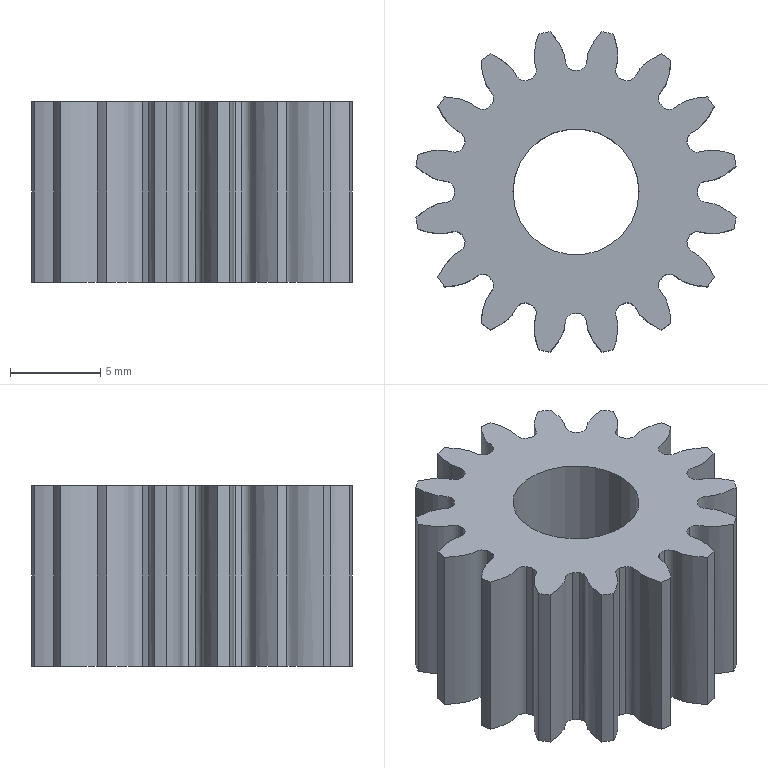Part | SolidWorks | features ICE 2, CirPattern 1, Extrusion 1, RefAxis 1 | 1 solid | 68 faces | box 17.771 x 17.771 x 10 mm | volume 1584 mm3 | cylinder 34 | spline 32 | plane 2 | commonest cylinder face diameters 13.5 x16 18 x16 7 x2